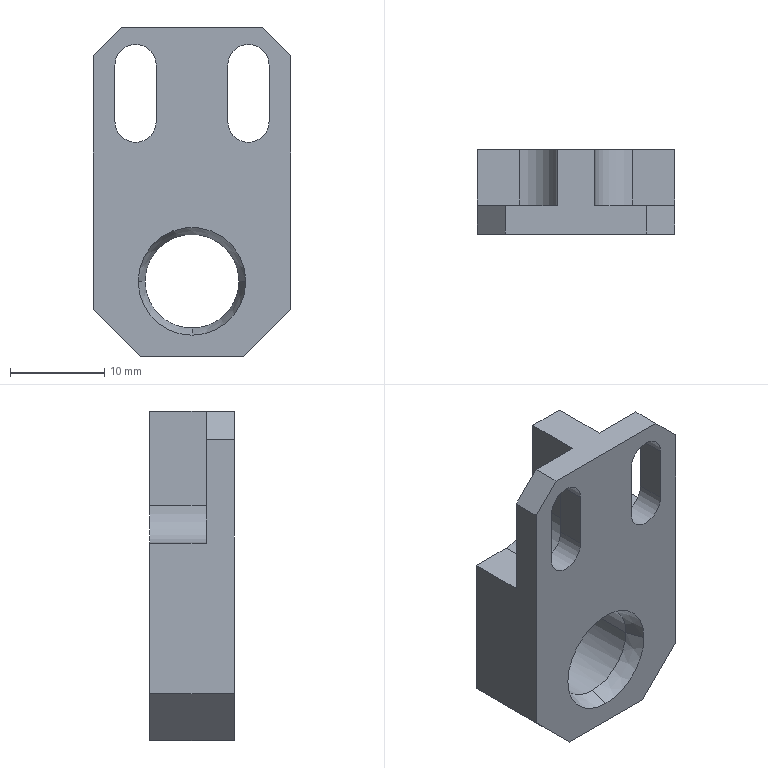Part | STEP file | 1519D1D1-5.stp.STEP | 1 solid | 31 faces | box 21 x 9 x 35 mm | volume 3996 mm3 | plane 20 | cylinder 8 | cone 3 | commonest cylinder face diameters 4.4 x4 8 x2 10 x2
STEP:
#1=CARTESIAN_POINT('',(-8.2,0.,-10.));
#2=VERTEX_POINT('',#1);
#3=CARTESIAN_POINT('',(-8.2,0.,-4.));
#4=VERTEX_POINT('',#3);
#5=CARTESIAN_POINT('',(-8.2,0.,-10.));
#6=DIRECTION('',(0.,0.,1.));
#7=VECTOR('',#6,1000.);
#8=LINE('',#5,#7);
#9=EDGE_CURVE('',#2,#4,#8,.T.);
#10=ORIENTED_EDGE('',*,*,#9,.T.);
#11=CARTESIAN_POINT('',(-3.8,0.,-4.));
#12=VERTEX_POINT('',#11);
#13=CARTESIAN_POINT('',(-6.,0.,-4.));
#14=DIRECTION('',(0.,1.,0.));
#15=DIRECTION('',(-1.,0.,0.));
#16=AXIS2_PLACEMENT_3D('',#13,#14,#15);
#17=CIRCLE('',#16,2.2);
#18=EDGE_CURVE('',#4,#12,#17,.T.);
#19=ORIENTED_EDGE('',*,*,#18,.T.);
#20=CARTESIAN_POINT('',(-3.8,0.,-10.));
#21=VERTEX_POINT('',#20);
#22=CARTESIAN_POINT('',(-3.8,0.,-4.));
#23=DIRECTION('',(0.,0.,-1.));
#24=VECTOR('',#23,1000.);
#25=LINE('',#22,#24);
#26=EDGE_CURVE('',#12,#21,#25,.T.);
#27=ORIENTED_EDGE('',*,*,#26,.T.);
#28=CARTESIAN_POINT('',(-6.,0.,-10.));
#29=DIRECTION('',(0.,1.,0.));
#30=DIRECTION('',(1.,0.,0.));
#31=AXIS2_PLACEMENT_3D('',#28,#29,#30);
#32=CIRCLE('',#31,2.2);
#33=EDGE_CURVE('',#21,#2,#32,.T.);
#34=ORIENTED_EDGE('',*,*,#33,.T.);
#35=EDGE_LOOP('',(#10,#19,#27,#34));
#36=FACE_BOUND('',#35,.T.);
#37=CARTESIAN_POINT('',(5.728,0.,-27.));
#38=VERTEX_POINT('',#37);
#39=CARTESIAN_POINT('',(0.,0.,-32.728));
#40=VERTEX_POINT('',#39);
#41=CARTESIAN_POINT('',(0.,0.,-27.));
#42=DIRECTION('',(0.,1.,0.));
#43=DIRECTION('',(1.,0.,0.));
#44=AXIS2_PLACEMENT_3D('',#41,#42,#43);
#45=CIRCLE('',#44,5.728);
#46=EDGE_CURVE('',#38,#40,#45,.T.);
#47=ORIENTED_EDGE('',*,*,#46,.T.);
#48=CARTESIAN_POINT('',(-5.728,0.,-27.));
#49=VERTEX_POINT('',#48);
#50=CARTESIAN_POINT('',(0.,0.,-27.));
#51=DIRECTION('',(0.,1.,0.));
#52=DIRECTION('',(1.,0.,0.));
#53=AXIS2_PLACEMENT_3D('',#50,#51,#52);
#54=CIRCLE('',#53,5.728);
#55=EDGE_CURVE('',#40,#49,#54,.T.);
#56=ORIENTED_EDGE('',*,*,#55,.T.);
#57=CARTESIAN_POINT('',(0.,0.,-27.));
#58=DIRECTION('',(0.,1.,0.));
#59=DIRECTION('',(-1.,0.,0.));
#60=AXIS2_PLACEMENT_3D('',#57,#58,#59);
#61=CIRCLE('',#60,5.728);
#62=EDGE_CURVE('',#49,#38,#61,.T.);
#63=ORIENTED_EDGE('',*,*,#62,.T.);
#64=EDGE_LOOP('',(#47,#56,#63));
#65=FACE_BOUND('',#64,.T.);
#66=CARTESIAN_POINT('',(3.8,0.,-4.));
#67=VERTEX_POINT('',#66);
#68=CARTESIAN_POINT('',(8.2,0.,-4.));
#69=VERTEX_POINT('',#68);
#70=CARTESIAN_POINT('',(6.,0.,-4.));
#71=DIRECTION('',(0.,1.,0.));
#72=DIRECTION('',(-1.,0.,0.));
#73=AXIS2_PLACEMENT_3D('',#70,#71,#72);
#74=CIRCLE('',#73,2.2);
#75=EDGE_CURVE('',#67,#69,#74,.T.);
#76=ORIENTED_EDGE('',*,*,#75,.T.);
#77=CARTESIAN_POINT('',(8.2,0.,-10.));
#78=VERTEX_POINT('',#77);
#79=CARTESIAN_POINT('',(8.2,0.,-4.));
#80=DIRECTION('',(0.,0.,-1.));
#81=VECTOR('',#80,1000.);
#82=LINE('',#79,#81);
#83=EDGE_CURVE('',#69,#78,#82,.T.);
#84=ORIENTED_EDGE('',*,*,#83,.T.);
#85=CARTESIAN_POINT('',(3.8,0.,-10.));
#86=VERTEX_POINT('',#85);
#87=CARTESIAN_POINT('',(6.,0.,-10.));
#88=DIRECTION('',(0.,1.,0.));
#89=DIRECTION('',(1.,0.,0.));
#90=AXIS2_PLACEMENT_3D('',#87,#88,#89);
#91=CIRCLE('',#90,2.2);
#92=EDGE_CURVE('',#78,#86,#91,.T.);
#93=ORIENTED_EDGE('',*,*,#92,.T.);
#94=CARTESIAN_POINT('',(3.8,0.,-10.));
#95=DIRECTION('',(0.,0.,1.));
#96=VECTOR('',#95,1000.);
#97=LINE('',#94,#96);
#98=EDGE_CURVE('',#86,#67,#97,.T.);
#99=ORIENTED_EDGE('',*,*,#98,.T.);
#100=EDGE_LOOP('',(#76,#84,#93,#99));
#101=FACE_BOUND('',#100,.T.);
#102=CARTESIAN_POINT('',(5.5,0.,-35.));
#103=VERTEX_POINT('',#102);
#104=CARTESIAN_POINT('',(-5.5,0.,-35.));
#105=VERTEX_POINT('',#104);
#106=CARTESIAN_POINT('',(5.5,0.,-35.));
#107=DIRECTION('',(-1.,0.,0.));
#108=VECTOR('',#107,1000.);
#109=LINE('',#106,#108);
#110=EDGE_CURVE('',#103,#105,#109,.T.);
#111=ORIENTED_EDGE('',*,*,#110,.F.);
#112=CARTESIAN_POINT('',(10.5,0.,-30.));
#113=VERTEX_POINT('',#112);
#114=CARTESIAN_POINT('',(5.5,0.,-35.));
#115=DIRECTION('',(0.7071,0.,0.7071));
#116=VECTOR('',#115,1000.);
#117=LINE('',#114,#116);
#118=EDGE_CURVE('',#103,#113,#117,.T.);
#119=ORIENTED_EDGE('',*,*,#118,.T.);
#120=CARTESIAN_POINT('',(10.5,0.,-3.));
#121=VERTEX_POINT('',#120);
#122=CARTESIAN_POINT('',(10.5,0.,-3.));
#123=DIRECTION('',(0.,0.,-1.));
#124=VECTOR('',#123,1000.);
#125=LINE('',#122,#124);
#126=EDGE_CURVE('',#121,#113,#125,.T.);
#127=ORIENTED_EDGE('',*,*,#126,.F.);
#128=CARTESIAN_POINT('',(7.5,0.,0.));
#129=VERTEX_POINT('',#128);
#130=CARTESIAN_POINT('',(10.5,0.,-3.));
#131=DIRECTION('',(-0.7071,0.,0.7071));
#132=VECTOR('',#131,1000.);
#133=LINE('',#130,#132);
#134=EDGE_CURVE('',#121,#129,#133,.T.);
#135=ORIENTED_EDGE('',*,*,#134,.T.);
#136=CARTESIAN_POINT('',(-7.5,0.,0.));
#137=VERTEX_POINT('',#136);
#138=CARTESIAN_POINT('',(-7.5,0.,0.));
#139=DIRECTION('',(1.,0.,0.));
#140=VECTOR('',#139,1000.);
#141=LINE('',#138,#140);
#142=EDGE_CURVE('',#137,#129,#141,.T.);
#143=ORIENTED_EDGE('',*,*,#142,.F.);
#144=CARTESIAN_POINT('',(-10.5,0.,-3.));
#145=VERTEX_POINT('',#144);
#146=CARTESIAN_POINT('',(-7.5,0.,0.));
#147=DIRECTION('',(-0.7071,0.,-0.7071));
#148=VECTOR('',#147,1000.);
#149=LINE('',#146,#148);
#150=EDGE_CURVE('',#137,#145,#149,.T.);
#151=ORIENTED_EDGE('',*,*,#150,.T.);
#152=CARTESIAN_POINT('',(-10.5,0.,-30.));
#153=VERTEX_POINT('',#152);
#154=CARTESIAN_POINT('',(-10.5,0.,-30.));
#155=DIRECTION('',(0.,0.,1.));
#156=VECTOR('',#155,1000.);
#157=LINE('',#154,#156);
#158=EDGE_CURVE('',#153,#145,#157,.T.);
#159=ORIENTED_EDGE('',*,*,#158,.F.);
#160=CARTESIAN_POINT('',(-10.5,0.,-30.));
#161=DIRECTION('',(0.7071,0.,-0.7071));
#162=VECTOR('',#161,1000.);
#163=LINE('',#160,#162);
#164=EDGE_CURVE('',#153,#105,#163,.T.);
#165=ORIENTED_EDGE('',*,*,#164,.T.);
#166=EDGE_LOOP('',(#111,#119,#127,#135,#143,#151,#159,#165));
#167=FACE_OUTER_BOUND('',#166,.T.);
#168=CARTESIAN_POINT('',(0.,0.,0.));
#169=DIRECTION('',(0.,1.,0.));
#170=DIRECTION('',(1.,0.,0.));
#171=AXIS2_PLACEMENT_3D('',#168,#169,#170);
#172=PLANE('',#171);
#173=ADVANCED_FACE('',(#36,#65,#101,#167),#172,.F.);
#174=CARTESIAN_POINT('',(3.8,3.,-4.));
#175=VERTEX_POINT('',#174);
#176=CARTESIAN_POINT('',(3.8,3.,-4.));
#177=DIRECTION('',(0.,-1.,0.));
#178=VECTOR('',#177,1000.);
#179=LINE('',#176,#178);
#180=EDGE_CURVE('',#175,#67,#179,.T.);
#181=ORIENTED_EDGE('',*,*,#180,.T.);
#182=ORIENTED_EDGE('',*,*,#98,.F.);
#183=CARTESIAN_POINT('',(3.8,3.,-10.));
#184=VERTEX_POINT('',#183);
#185=CARTESIAN_POINT('',(3.8,3.,-10.));
#186=DIRECTION('',(0.,-1.,0.));
#187=VECTOR('',#186,1000.);
#188=LINE('',#185,#187);
#189=EDGE_CURVE('',#184,#86,#188,.T.);
#190=ORIENTED_EDGE('',*,*,#189,.F.);
#191=CARTESIAN_POINT('',(3.8,3.,-10.));
#192=DIRECTION('',(0.,0.,1.));
#193=VECTOR('',#192,1000.);
#194=LINE('',#191,#193);
#195=EDGE_CURVE('',#184,#175,#194,.T.);
#196=ORIENTED_EDGE('',*,*,#195,.T.);
#197=EDGE_LOOP('',(#181,#182,#190,#196));
#198=FACE_OUTER_BOUND('',#197,.T.);
#199=CARTESIAN_POINT('',(3.8,9.,-10.));
#200=DIRECTION('',(-1.,0.,0.));
#201=DIRECTION('',(0.,0.,1.));
#202=AXIS2_PLACEMENT_3D('',#199,#200,#201);
#203=PLANE('',#202);
#204=ADVANCED_FACE('',(#198),#203,.F.);
#205=CARTESIAN_POINT('',(-3.8,3.,-4.));
#206=VERTEX_POINT('',#205);
#207=CARTESIAN_POINT('',(-3.8,3.,-10.));
#208=VERTEX_POINT('',#207);
#209=CARTESIAN_POINT('',(-3.8,3.,-4.));
#210=DIRECTION('',(0.,0.,-1.));
#211=VECTOR('',#210,1000.);
#212=LINE('',#209,#211);
#213=EDGE_CURVE('',#206,#208,#212,.T.);
#214=ORIENTED_EDGE('',*,*,#213,.F.);
#215=CARTESIAN_POINT('',(-8.2,3.,-4.));
#216=VERTEX_POINT('',#215);
#217=CARTESIAN_POINT('',(-6.,3.,-4.));
#218=DIRECTION('',(0.,1.,0.));
#219=DIRECTION('',(-1.,0.,0.));
#220=AXIS2_PLACEMENT_3D('',#217,#218,#219);
#221=CIRCLE('',#220,2.2);
#222=EDGE_CURVE('',#216,#206,#221,.T.);
#223=ORIENTED_EDGE('',*,*,#222,.F.);
#224=CARTESIAN_POINT('',(-8.2,3.,-10.));
#225=VERTEX_POINT('',#224);
#226=CARTESIAN_POINT('',(-8.2,3.,-10.));
#227=DIRECTION('',(0.,0.,1.));
#228=VECTOR('',#227,1000.);
#229=LINE('',#226,#228);
#230=EDGE_CURVE('',#225,#216,#229,.T.);
#231=ORIENTED_EDGE('',*,*,#230,.F.);
#232=CARTESIAN_POINT('',(-6.,3.,-10.));
#233=DIRECTION('',(0.,1.,0.));
#234=DIRECTION('',(1.,0.,0.));
#235=AXIS2_PLACEMENT_3D('',#232,#233,#234);
#236=CIRCLE('',#235,2.2);
#237=EDGE_CURVE('',#208,#225,#236,.T.);
#238=ORIENTED_EDGE('',*,*,#237,.F.);
#239=EDGE_LOOP('',(#214,#223,#231,#238));
#240=FACE_BOUND('',#239,.T.);
#241=CARTESIAN_POINT('',(-7.5,3.,0.));
#242=VERTEX_POINT('',#241);
#243=CARTESIAN_POINT('',(-2.,3.,0.));
#244=VERTEX_POINT('',#243);
#245=CARTESIAN_POINT('',(-7.5,3.,0.));
#246=DIRECTION('',(1.,0.,0.));
#247=VECTOR('',#246,1000.);
#248=LINE('',#245,#247);
#249=EDGE_CURVE('',#242,#244,#248,.T.);
#250=ORIENTED_EDGE('',*,*,#249,.T.);
#251=CARTESIAN_POINT('',(-2.,3.,-10.));
#252=VERTEX_POINT('',#251);
#253=CARTESIAN_POINT('',(-2.,3.,0.));
#254=DIRECTION('',(0.,0.,-1.));
#255=VECTOR('',#254,1000.);
#256=LINE('',#253,#255);
#257=EDGE_CURVE('',#244,#252,#256,.T.);
#258=ORIENTED_EDGE('',*,*,#257,.T.);
#259=CARTESIAN_POINT('',(-6.,3.,-14.));
#260=VERTEX_POINT('',#259);
#261=CARTESIAN_POINT('',(-6.,3.,-10.));
#262=DIRECTION('',(0.,1.,0.));
#263=DIRECTION('',(1.,0.,0.));
#264=AXIS2_PLACEMENT_3D('',#261,#262,#263);
#265=CIRCLE('',#264,4.);
#266=EDGE_CURVE('',#252,#260,#265,.T.);
#267=ORIENTED_EDGE('',*,*,#266,.T.);
#268=CARTESIAN_POINT('',(-10.5,3.,-14.));
#269=VERTEX_POINT('',#268);
#270=CARTESIAN_POINT('',(-6.,3.,-14.));
#271=DIRECTION('',(-1.,0.,0.));
#272=VECTOR('',#271,1000.);
#273=LINE('',#270,#272);
#274=EDGE_CURVE('',#260,#269,#273,.T.);
#275=ORIENTED_EDGE('',*,*,#274,.T.);
#276=CARTESIAN_POINT('',(-10.5,3.,-3.));
#277=VERTEX_POINT('',#276);
#278=CARTESIAN_POINT('',(-10.5,3.,-3.));
#279=DIRECTION('',(0.,0.,-1.));
#280=VECTOR('',#279,1000.);
#281=LINE('',#278,#280);
#282=EDGE_CURVE('',#277,#269,#281,.T.);
#283=ORIENTED_EDGE('',*,*,#282,.F.);
#284=CARTESIAN_POINT('',(-10.5,3.,-3.));
#285=DIRECTION('',(0.7071,0.,0.7071));
#286=VECTOR('',#285,1000.);
#287=LINE('',#284,#286);
#288=EDGE_CURVE('',#277,#242,#287,.T.);
#289=ORIENTED_EDGE('',*,*,#288,.T.);
#290=EDGE_LOOP('',(#250,#258,#267,#275,#283,#289));
#291=FACE_OUTER_BOUND('',#290,.T.);
#292=CARTESIAN_POINT('',(0.,3.,0.));
#293=DIRECTION('',(0.,1.,0.));
#294=DIRECTION('',(1.,0.,0.));
#295=AXIS2_PLACEMENT_3D('',#292,#293,#294);
#296=PLANE('',#295);
#297=ADVANCED_FACE('',(#240,#291),#296,.T.);
#298=CARTESIAN_POINT('',(8.2,3.,-10.));
#299=VERTEX_POINT('',#298);
#300=CARTESIAN_POINT('',(6.,3.,-10.));
#301=DIRECTION('',(0.,1.,0.));
#302=DIRECTION('',(1.,0.,0.));
#303=AXIS2_PLACEMENT_3D('',#300,#301,#302);
#304=CIRCLE('',#303,2.2);
#305=EDGE_CURVE('',#299,#184,#304,.T.);
#306=ORIENTED_EDGE('',*,*,#305,.F.);
#307=CARTESIAN_POINT('',(8.2,3.,-4.));
#308=VERTEX_POINT('',#307);
#309=CARTESIAN_POINT('',(8.2,3.,-4.));
#310=DIRECTION('',(0.,0.,-1.));
#311=VECTOR('',#310,1000.);
#312=LINE('',#309,#311);
#313=EDGE_CURVE('',#308,#299,#312,.T.);
#314=ORIENTED_EDGE('',*,*,#313,.F.);
#315=CARTESIAN_POINT('',(6.,3.,-4.));
#316=DIRECTION('',(0.,1.,0.));
#317=DIRECTION('',(-1.,0.,0.));
#318=AXIS2_PLACEMENT_3D('',#315,#316,#317);
#319=CIRCLE('',#318,2.2);
#320=EDGE_CURVE('',#175,#308,#319,.T.);
#321=ORIENTED_EDGE('',*,*,#320,.F.);
#322=ORIENTED_EDGE('',*,*,#195,.F.);
#323=EDGE_LOOP('',(#306,#314,#321,#322));
#324=FACE_BOUND('',#323,.T.);
#325=CARTESIAN_POINT('',(10.5,3.,-3.));
#326=VERTEX_POINT('',#325);
#327=CARTESIAN_POINT('',(10.5,3.,-14.));
#328=VERTEX_POINT('',#327);
#329=CARTESIAN_POINT('',(10.5,3.,-3.));
#330=DIRECTION('',(0.,0.,-1.));
#331=VECTOR('',#330,1000.);
#332=LINE('',#329,#331);
#333=EDGE_CURVE('',#326,#328,#332,.T.);
#334=ORIENTED_EDGE('',*,*,#333,.T.);
#335=CARTESIAN_POINT('',(6.,3.,-14.));
#336=VERTEX_POINT('',#335);
#337=CARTESIAN_POINT('',(10.5,3.,-14.));
#338=DIRECTION('',(-1.,0.,0.));
#339=VECTOR('',#338,1000.);
#340=LINE('',#337,#339);
#341=EDGE_CURVE('',#328,#336,#340,.T.);
#342=ORIENTED_EDGE('',*,*,#341,.T.);
#343=CARTESIAN_POINT('',(2.,3.,-10.));
#344=VERTEX_POINT('',#343);
#345=CARTESIAN_POINT('',(6.,3.,-10.));
#346=DIRECTION('',(0.,1.,0.));
#347=DIRECTION('',(0.,0.,-1.));
#348=AXIS2_PLACEMENT_3D('',#345,#346,#347);
#349=CIRCLE('',#348,4.);
#350=EDGE_CURVE('',#336,#344,#349,.T.);
#351=ORIENTED_EDGE('',*,*,#350,.T.);
#352=CARTESIAN_POINT('',(2.,3.,0.));
#353=VERTEX_POINT('',#352);
#354=CARTESIAN_POINT('',(2.,3.,-10.));
#355=DIRECTION('',(0.,0.,1.));
#356=VECTOR('',#355,1000.);
#357=LINE('',#354,#356);
#358=EDGE_CURVE('',#344,#353,#357,.T.);
#359=ORIENTED_EDGE('',*,*,#358,.T.);
#360=CARTESIAN_POINT('',(7.5,3.,0.));
#361=VERTEX_POINT('',#360);
#362=CARTESIAN_POINT('',(2.,3.,0.));
#363=DIRECTION('',(1.,0.,0.));
#364=VECTOR('',#363,1000.);
#365=LINE('',#362,#364);
#366=EDGE_CURVE('',#353,#361,#365,.T.);
#367=ORIENTED_EDGE('',*,*,#366,.T.);
#368=CARTESIAN_POINT('',(7.5,3.,0.));
#369=DIRECTION('',(0.7071,0.,-0.7071));
#370=VECTOR('',#369,1000.);
#371=LINE('',#368,#370);
#372=EDGE_CURVE('',#361,#326,#371,.T.);
#373=ORIENTED_EDGE('',*,*,#372,.T.);
#374=EDGE_LOOP('',(#334,#342,#351,#359,#367,#373));
#375=FACE_OUTER_BOUND('',#374,.T.);
#376=CARTESIAN_POINT('',(0.,3.,0.));
#377=DIRECTION('',(0.,1.,0.));
#378=DIRECTION('',(1.,0.,0.));
#379=AXIS2_PLACEMENT_3D('',#376,#377,#378);
#380=PLANE('',#379);
#381=ADVANCED_FACE('',(#324,#375),#380,.T.);
#382=CARTESIAN_POINT('',(-8.2,3.,-10.));
#383=DIRECTION('',(0.,-1.,0.));
#384=VECTOR('',#383,1000.);
#385=LINE('',#382,#384);
#386=EDGE_CURVE('',#225,#2,#385,.T.);
#387=ORIENTED_EDGE('',*,*,#386,.T.);
#388=ORIENTED_EDGE('',*,*,#33,.F.);
#389=CARTESIAN_POINT('',(-3.8,3.,-10.));
#390=DIRECTION('',(0.,-1.,0.));
#391=VECTOR('',#390,1000.);
#392=LINE('',#389,#391);
#393=EDGE_CURVE('',#208,#21,#392,.T.);
#394=ORIENTED_EDGE('',*,*,#393,.F.);
#395=ORIENTED_EDGE('',*,*,#237,.T.);
#396=EDGE_LOOP('',(#387,#388,#394,#395));
#397=FACE_OUTER_BOUND('',#396,.T.);
#398=CARTESIAN_POINT('',(-6.,9.,-10.));
#399=DIRECTION('',(0.,1.,0.));
#400=DIRECTION('',(1.,0.,0.));
#401=AXIS2_PLACEMENT_3D('',#398,#399,#400);
#402=CYLINDRICAL_SURFACE('',#401,2.2);
#403=ADVANCED_FACE('',(#397),#402,.F.);
#404=ORIENTED_EDGE('',*,*,#393,.T.);
#405=ORIENTED_EDGE('',*,*,#26,.F.);
#406=CARTESIAN_POINT('',(-3.8,3.,-4.));
#407=DIRECTION('',(0.,-1.,0.));
#408=VECTOR('',#407,1000.);
#409=LINE('',#406,#408);
#410=EDGE_CURVE('',#206,#12,#409,.T.);
#411=ORIENTED_EDGE('',*,*,#410,.F.);
#412=ORIENTED_EDGE('',*,*,#213,.T.);
#413=EDGE_LOOP('',(#404,#405,#411,#412));
#414=FACE_OUTER_BOUND('',#413,.T.);
#415=CARTESIAN_POINT('',(-3.8,9.,-4.));
#416=DIRECTION('',(1.,0.,0.));
#417=DIRECTION('',(0.,1.,0.));
#418=AXIS2_PLACEMENT_3D('',#415,#416,#417);
#419=PLANE('',#418);
#420=ADVANCED_FACE('',(#414),#419,.F.);
#421=ORIENTED_EDGE('',*,*,#410,.T.);
#422=ORIENTED_EDGE('',*,*,#18,.F.);
#423=CARTESIAN_POINT('',(-8.2,3.,-4.));
#424=DIRECTION('',(0.,-1.,0.));
#425=VECTOR('',#424,1000.);
#426=LINE('',#423,#425);
#427=EDGE_CURVE('',#216,#4,#426,.T.);
#428=ORIENTED_EDGE('',*,*,#427,.F.);
#429=ORIENTED_EDGE('',*,*,#222,.T.);
#430=EDGE_LOOP('',(#421,#422,#428,#429));
#431=FACE_OUTER_BOUND('',#430,.T.);
#432=CARTESIAN_POINT('',(-6.,9.,-4.));
#433=DIRECTION('',(0.,1.,0.));
#434=DIRECTION('',(1.,0.,0.));
#435=AXIS2_PLACEMENT_3D('',#432,#433,#434);
#436=CYLINDRICAL_SURFACE('',#435,2.2);
#437=ADVANCED_FACE('',(#431),#436,.F.);
#438=ORIENTED_EDGE('',*,*,#427,.T.);
#439=ORIENTED_EDGE('',*,*,#9,.F.);
#440=ORIENTED_EDGE('',*,*,#386,.F.);
#441=ORIENTED_EDGE('',*,*,#230,.T.);
#442=EDGE_LOOP('',(#438,#439,#440,#441));
#443=FACE_OUTER_BOUND('',#442,.T.);
#444=CARTESIAN_POINT('',(-8.2,9.,-10.));
#445=DIRECTION('',(-1.,0.,0.));
#446=DIRECTION('',(0.,0.,1.));
#447=AXIS2_PLACEMENT_3D('',#444,#445,#446);
#448=PLANE('',#447);
#449=ADVANCED_FACE('',(#443),#448,.F.);
#450=CARTESIAN_POINT('',(8.2,3.,-4.));
#451=DIRECTION('',(0.,-1.,0.));
#452=VECTOR('',#451,1000.);
#453=LINE('',#450,#452);
#454=EDGE_CURVE('',#308,#69,#453,.T.);
#455=ORIENTED_EDGE('',*,*,#454,.T.);
#456=ORIENTED_EDGE('',*,*,#75,.F.);
#457=ORIENTED_EDGE('',*,*,#180,.F.);
#458=ORIENTED_EDGE('',*,*,#320,.T.);
#459=EDGE_LOOP('',(#455,#456,#457,#458));
#460=FACE_OUTER_BOUND('',#459,.T.);
#461=CARTESIAN_POINT('',(6.,9.,-4.));
#462=DIRECTION('',(0.,1.,0.));
#463=DIRECTION('',(1.,0.,0.));
#464=AXIS2_PLACEMENT_3D('',#461,#462,#463);
#465=CYLINDRICAL_SURFACE('',#464,2.2);
#466=ADVANCED_FACE('',(#460),#465,.F.);
#467=CARTESIAN_POINT('',(8.2,3.,-10.));
#468=DIRECTION('',(0.,-1.,0.));
#469=VECTOR('',#468,1000.);
#470=LINE('',#467,#469);
#471=EDGE_CURVE('',#299,#78,#470,.T.);
#472=ORIENTED_EDGE('',*,*,#471,.T.);
#473=ORIENTED_EDGE('',*,*,#83,.F.);
#474=ORIENTED_EDGE('',*,*,#454,.F.);
#475=ORIENTED_EDGE('',*,*,#313,.T.);
#476=EDGE_LOOP('',(#472,#473,#474,#475));
#477=FACE_OUTER_BOUND('',#476,.T.);
#478=CARTESIAN_POINT('',(8.2,9.,-4.));
#479=DIRECTION('',(1.,0.,0.));
#480=DIRECTION('',(0.,1.,0.));
#481=AXIS2_PLACEMENT_3D('',#478,#479,#480);
#482=PLANE('',#481);
#483=ADVANCED_FACE('',(#477),#482,.F.);
#484=ORIENTED_EDGE('',*,*,#189,.T.);
#485=ORIENTED_EDGE('',*,*,#92,.F.);
#486=ORIENTED_EDGE('',*,*,#471,.F.);
#487=ORIENTED_EDGE('',*,*,#305,.T.);
#488=EDGE_LOOP('',(#484,#485,#486,#487));
#489=FACE_OUTER_BOUND('',#488,.T.);
#490=CARTESIAN_POINT('',(6.,9.,-10.));
#491=DIRECTION('',(0.,1.,0.));
#492=DIRECTION('',(1.,0.,0.));
#493=AXIS2_PLACEMENT_3D('',#490,#491,#492);
#494=CYLINDRICAL_SURFACE('',#493,2.2);
#495=ADVANCED_FACE('',(#489),#494,.F.);
#496=CARTESIAN_POINT('',(-7.5,3.,0.));
#497=DIRECTION('',(0.,-1.,0.));
#498=VECTOR('',#497,1000.);
#499=LINE('',#496,#498);
#500=EDGE_CURVE('',#242,#137,#499,.T.);
#501=ORIENTED_EDGE('',*,*,#500,.F.);
#502=ORIENTED_EDGE('',*,*,#288,.F.);
#503=CARTESIAN_POINT('',(-10.5,3.,-3.));
#504=DIRECTION('',(0.,-1.,0.));
#505=VECTOR('',#504,1000.);
#506=LINE('',#503,#505);
#507=EDGE_CURVE('',#277,#145,#506,.T.);
#508=ORIENTED_EDGE('',*,*,#507,.T.);
#509=ORIENTED_EDGE('',*,*,#150,.F.);
#510=EDGE_LOOP('',(#501,#502,#508,#509));
#511=FACE_OUTER_BOUND('',#510,.T.);
#512=CARTESIAN_POINT('',(-9.,1.5,-1.5));
#513=DIRECTION('',(-0.7071,0.,0.7071));
#514=DIRECTION('',(0.,1.,0.));
#515=AXIS2_PLACEMENT_3D('',#512,#513,#514);
#516=PLANE('',#515);
#517=ADVANCED_FACE('',(#511),#516,.T.);
#518=ORIENTED_EDGE('',*,*,#158,.T.);
#519=ORIENTED_EDGE('',*,*,#507,.F.);
#520=ORIENTED_EDGE('',*,*,#282,.T.);
#521=CARTESIAN_POINT('',(-10.5,9.,-14.));
#522=VERTEX_POINT('',#521);
#523=CARTESIAN_POINT('',(-10.5,9.,-14.));
#524=DIRECTION('',(0.,-1.,0.));
#525=VECTOR('',#524,1000.);
#526=LINE('',#523,#525);
#527=EDGE_CURVE('',#522,#269,#526,.T.);
#528=ORIENTED_EDGE('',*,*,#527,.F.);
#529=CARTESIAN_POINT('',(-10.5,9.,-30.));
#530=VERTEX_POINT('',#529);
#531=CARTESIAN_POINT('',(-10.5,9.,-30.));
#532=DIRECTION('',(0.,0.,1.));
#533=VECTOR('',#532,1000.);
#534=LINE('',#531,#533);
#535=EDGE_CURVE('',#530,#522,#534,.T.);
#536=ORIENTED_EDGE('',*,*,#535,.F.);
#537=CARTESIAN_POINT('',(-10.5,9.,-30.));
#538=DIRECTION('',(0.,-1.,0.));
#539=VECTOR('',#538,1000.);
#540=LINE('',#537,#539);
#541=EDGE_CURVE('',#530,#153,#540,.T.);
#542=ORIENTED_EDGE('',*,*,#541,.T.);
#543=EDGE_LOOP('',(#518,#519,#520,#528,#536,#542));
#544=FACE_OUTER_BOUND('',#543,.T.);
#545=CARTESIAN_POINT('',(-10.5,0.,-35.));
#546=DIRECTION('',(-1.,0.,0.));
#547=DIRECTION('',(0.,0.,1.));
#548=AXIS2_PLACEMENT_3D('',#545,#546,#547);
#549=PLANE('',#548);
#550=ADVANCED_FACE('',(#544),#549,.T.);
#551=ORIENTED_EDGE('',*,*,#541,.F.);
#552=CARTESIAN_POINT('',(-5.5,9.,-35.));
#553=VERTEX_POINT('',#552);
#554=CARTESIAN_POINT('',(-5.5,9.,-35.));
#555=DIRECTION('',(-0.7071,0.,0.7071));
#556=VECTOR('',#555,1000.);
#557=LINE('',#554,#556);
#558=EDGE_CURVE('',#553,#530,#557,.T.);
#559=ORIENTED_EDGE('',*,*,#558,.F.);
#560=CARTESIAN_POINT('',(-5.5,9.,-35.));
#561=DIRECTION('',(0.,-1.,0.));
#562=VECTOR('',#561,1000.);
#563=LINE('',#560,#562);
#564=EDGE_CURVE('',#553,#105,#563,.T.);
#565=ORIENTED_EDGE('',*,*,#564,.T.);
#566=ORIENTED_EDGE('',*,*,#164,.F.);
#567=EDGE_LOOP('',(#551,#559,#565,#566));
#568=FACE_OUTER_BOUND('',#567,.T.);
#569=CARTESIAN_POINT('',(-8.,4.5,-32.5));
#570=DIRECTION('',(-0.7071,0.,-0.7071));
#571=DIRECTION('',(-0.7071,0.,0.7071));
#572=AXIS2_PLACEMENT_3D('',#569,#570,#571);
#573=PLANE('',#572);
#574=ADVANCED_FACE('',(#568),#573,.T.);
#575=CARTESIAN_POINT('',(5.5,9.,-35.));
#576=VERTEX_POINT('',#575);
#577=CARTESIAN_POINT('',(5.5,9.,-35.));
#578=DIRECTION('',(-1.,0.,0.));
#579=VECTOR('',#578,1000.);
#580=LINE('',#577,#579);
#581=EDGE_CURVE('',#576,#553,#580,.T.);
#582=ORIENTED_EDGE('',*,*,#581,.F.);
#583=CARTESIAN_POINT('',(5.5,9.,-35.));
#584=DIRECTION('',(0.,-1.,0.));
#585=VECTOR('',#584,1000.);
#586=LINE('',#583,#585);
#587=EDGE_CURVE('',#576,#103,#586,.T.);
#588=ORIENTED_EDGE('',*,*,#587,.T.);
#589=ORIENTED_EDGE('',*,*,#110,.T.);
#590=ORIENTED_EDGE('',*,*,#564,.F.);
#591=EDGE_LOOP('',(#582,#588,#589,#590));
#592=FACE_OUTER_BOUND('',#591,.T.);
#593=CARTESIAN_POINT('',(10.5,0.,-35.));
#594=DIRECTION('',(0.,0.,-1.));
#595=DIRECTION('',(0.,-1.,0.));
#596=AXIS2_PLACEMENT_3D('',#593,#594,#595);
#597=PLANE('',#596);
#598=ADVANCED_FACE('',(#592),#597,.T.);
#599=ORIENTED_EDGE('',*,*,#587,.F.);
#600=CARTESIAN_POINT('',(10.5,9.,-30.));
#601=VERTEX_POINT('',#600);
#602=CARTESIAN_POINT('',(10.5,9.,-30.));
#603=DIRECTION('',(-0.7071,0.,-0.7071));
#604=VECTOR('',#603,1000.);
#605=LINE('',#602,#604);
#606=EDGE_CURVE('',#601,#576,#605,.T.);
#607=ORIENTED_EDGE('',*,*,#606,.F.);
#608=CARTESIAN_POINT('',(10.5,9.,-30.));
#609=DIRECTION('',(0.,-1.,0.));
#610=VECTOR('',#609,1000.);
#611=LINE('',#608,#610);
#612=EDGE_CURVE('',#601,#113,#611,.T.);
#613=ORIENTED_EDGE('',*,*,#612,.T.);
#614=ORIENTED_EDGE('',*,*,#118,.F.);
#615=EDGE_LOOP('',(#599,#607,#613,#614));
#616=FACE_OUTER_BOUND('',#615,.T.);
#617=CARTESIAN_POINT('',(8.,4.5,-32.5));
#618=DIRECTION('',(0.7071,0.,-0.7071));
#619=DIRECTION('',(0.,-1.,0.));
#620=AXIS2_PLACEMENT_3D('',#617,#618,#619);
#621=PLANE('',#620);
#622=ADVANCED_FACE('',(#616),#621,.T.);
#623=CARTESIAN_POINT('',(10.5,9.,-14.));
#624=VERTEX_POINT('',#623);
#625=CARTESIAN_POINT('',(10.5,9.,-14.));
#626=DIRECTION('',(0.,0.,-1.));
#627=VECTOR('',#626,1000.);
#628=LINE('',#625,#627);
#629=EDGE_CURVE('',#624,#601,#628,.T.);
#630=ORIENTED_EDGE('',*,*,#629,.F.);
#631=CARTESIAN_POINT('',(10.5,9.,-14.));
#632=DIRECTION('',(0.,-1.,0.));
#633=VECTOR('',#632,1000.);
#634=LINE('',#631,#633);
#635=EDGE_CURVE('',#624,#328,#634,.T.);
#636=ORIENTED_EDGE('',*,*,#635,.T.);
#637=ORIENTED_EDGE('',*,*,#333,.F.);
#638=CARTESIAN_POINT('',(10.5,3.,-3.));
#639=DIRECTION('',(0.,-1.,0.));
#640=VECTOR('',#639,1000.);
#641=LINE('',#638,#640);
#642=EDGE_CURVE('',#326,#121,#641,.T.);
#643=ORIENTED_EDGE('',*,*,#642,.T.);
#644=ORIENTED_EDGE('',*,*,#126,.T.);
#645=ORIENTED_EDGE('',*,*,#612,.F.);
#646=EDGE_LOOP('',(#630,#636,#637,#643,#644,#645));
#647=FACE_OUTER_BOUND('',#646,.T.);
#648=CARTESIAN_POINT('',(10.5,0.,0.));
#649=DIRECTION('',(1.,0.,0.));
#650=DIRECTION('',(0.,1.,0.));
#651=AXIS2_PLACEMENT_3D('',#648,#649,#650);
#652=PLANE('',#651);
#653=ADVANCED_FACE('',(#647),#652,.T.);
#654=ORIENTED_EDGE('',*,*,#642,.F.);
#655=ORIENTED_EDGE('',*,*,#372,.F.);
#656=CARTESIAN_POINT('',(7.5,3.,0.));
#657=DIRECTION('',(0.,-1.,0.));
#658=VECTOR('',#657,1000.);
#659=LINE('',#656,#658);
#660=EDGE_CURVE('',#361,#129,#659,.T.);
#661=ORIENTED_EDGE('',*,*,#660,.T.);
#662=ORIENTED_EDGE('',*,*,#134,.F.);
#663=EDGE_LOOP('',(#654,#655,#661,#662));
#664=FACE_OUTER_BOUND('',#663,.T.);
#665=CARTESIAN_POINT('',(9.,1.5,-1.5));
#666=DIRECTION('',(0.7071,0.,0.7071));
#667=DIRECTION('',(0.,-1.,0.));
#668=AXIS2_PLACEMENT_3D('',#665,#666,#667);
#669=PLANE('',#668);
#670=ADVANCED_FACE('',(#664),#669,.T.);
#671=ORIENTED_EDGE('',*,*,#142,.T.);
#672=ORIENTED_EDGE('',*,*,#660,.F.);
#673=ORIENTED_EDGE('',*,*,#366,.F.);
#674=CARTESIAN_POINT('',(2.,9.,0.));
#675=VERTEX_POINT('',#674);
#676=CARTESIAN_POINT('',(2.,9.,0.));
#677=DIRECTION('',(0.,-1.,0.));
#678=VECTOR('',#677,1000.);
#679=LINE('',#676,#678);
#680=EDGE_CURVE('',#675,#353,#679,.T.);
#681=ORIENTED_EDGE('',*,*,#680,.F.);
#682=CARTESIAN_POINT('',(-2.,9.,0.));
#683=VERTEX_POINT('',#682);
#684=CARTESIAN_POINT('',(-2.,9.,0.));
#685=DIRECTION('',(1.,0.,0.));
#686=VECTOR('',#685,1000.);
#687=LINE('',#684,#686);
#688=EDGE_CURVE('',#683,#675,#687,.T.);
#689=ORIENTED_EDGE('',*,*,#688,.F.);
#690=CARTESIAN_POINT('',(-2.,9.,0.));
#691=DIRECTION('',(0.,-1.,0.));
#692=VECTOR('',#691,1000.);
#693=LINE('',#690,#692);
#694=EDGE_CURVE('',#683,#244,#693,.T.);
#695=ORIENTED_EDGE('',*,*,#694,.T.);
#696=ORIENTED_EDGE('',*,*,#249,.F.);
#697=ORIENTED_EDGE('',*,*,#500,.T.);
#698=EDGE_LOOP('',(#671,#672,#673,#681,#689,#695,#696,#697));
#699=FACE_OUTER_BOUND('',#698,.T.);
#700=CARTESIAN_POINT('',(-10.5,0.,0.));
#701=DIRECTION('',(0.,0.,1.));
#702=DIRECTION('',(1.,0.,0.));
#703=AXIS2_PLACEMENT_3D('',#700,#701,#702);
#704=PLANE('',#703);
#705=ADVANCED_FACE('',(#699),#704,.T.);
#706=CARTESIAN_POINT('',(-2.,9.,-10.));
#707=VERTEX_POINT('',#706);
#708=CARTESIAN_POINT('',(-2.,9.,-10.));
#709=DIRECTION('',(0.,-1.,0.));
#710=VECTOR('',#709,1000.);
#711=LINE('',#708,#710);
#712=EDGE_CURVE('',#707,#252,#711,.T.);
#713=ORIENTED_EDGE('',*,*,#712,.T.);
#714=ORIENTED_EDGE('',*,*,#257,.F.);
#715=ORIENTED_EDGE('',*,*,#694,.F.);
#716=CARTESIAN_POINT('',(-2.,9.,0.));
#717=DIRECTION('',(0.,0.,-1.));
#718=VECTOR('',#717,1000.);
#719=LINE('',#716,#718);
#720=EDGE_CURVE('',#683,#707,#719,.T.);
#721=ORIENTED_EDGE('',*,*,#720,.T.);
#722=EDGE_LOOP('',(#713,#714,#715,#721));
#723=FACE_OUTER_BOUND('',#722,.T.);
#724=CARTESIAN_POINT('',(-2.,9.,0.));
#725=DIRECTION('',(1.,0.,0.));
#726=DIRECTION('',(0.,1.,0.));
#727=AXIS2_PLACEMENT_3D('',#724,#725,#726);
#728=PLANE('',#727);
#729=ADVANCED_FACE('',(#723),#728,.F.);
#730=CARTESIAN_POINT('',(-5.,9.,-27.));
#731=VERTEX_POINT('',#730);
#732=CARTESIAN_POINT('',(5.,9.,-27.));
#733=VERTEX_POINT('',#732);
#734=CARTESIAN_POINT('',(0.,9.,-27.));
#735=DIRECTION('',(0.,1.,0.));
#736=DIRECTION('',(-1.,0.,0.));
#737=AXIS2_PLACEMENT_3D('',#734,#735,#736);
#738=CIRCLE('',#737,5.);
#739=EDGE_CURVE('',#731,#733,#738,.T.);
#740=ORIENTED_EDGE('',*,*,#739,.F.);
#741=CARTESIAN_POINT('',(0.,9.,-27.));
#742=DIRECTION('',(0.,1.,0.));
#743=DIRECTION('',(1.,0.,0.));
#744=AXIS2_PLACEMENT_3D('',#741,#742,#743);
#745=CIRCLE('',#744,5.);
#746=EDGE_CURVE('',#733,#731,#745,.T.);
#747=ORIENTED_EDGE('',*,*,#746,.F.);
#748=EDGE_LOOP('',(#740,#747));
#749=FACE_BOUND('',#748,.T.);
#750=ORIENTED_EDGE('',*,*,#535,.T.);
#751=CARTESIAN_POINT('',(-6.,9.,-14.));
#752=VERTEX_POINT('',#751);
#753=CARTESIAN_POINT('',(-10.5,9.,-14.));
#754=DIRECTION('',(1.,0.,0.));
#755=VECTOR('',#754,1000.);
#756=LINE('',#753,#755);
#757=EDGE_CURVE('',#522,#752,#756,.T.);
#758=ORIENTED_EDGE('',*,*,#757,.T.);
#759=CARTESIAN_POINT('',(-6.,9.,-10.));
#760=DIRECTION('',(0.,1.,0.));
#761=DIRECTION('',(1.,0.,0.));
#762=AXIS2_PLACEMENT_3D('',#759,#760,#761);
#763=CIRCLE('',#762,4.);
#764=EDGE_CURVE('',#707,#752,#763,.T.);
#765=ORIENTED_EDGE('',*,*,#764,.F.);
#766=ORIENTED_EDGE('',*,*,#720,.F.);
#767=ORIENTED_EDGE('',*,*,#688,.T.);
#768=CARTESIAN_POINT('',(2.,9.,-10.));
#769=VERTEX_POINT('',#768);
#770=CARTESIAN_POINT('',(2.,9.,0.));
#771=DIRECTION('',(0.,0.,-1.));
#772=VECTOR('',#771,1000.);
#773=LINE('',#770,#772);
#774=EDGE_CURVE('',#675,#769,#773,.T.);
#775=ORIENTED_EDGE('',*,*,#774,.T.);
#776=CARTESIAN_POINT('',(6.,9.,-14.));
#777=VERTEX_POINT('',#776);
#778=CARTESIAN_POINT('',(6.,9.,-10.));
#779=DIRECTION('',(0.,1.,0.));
#780=DIRECTION('',(0.,0.,-1.));
#781=AXIS2_PLACEMENT_3D('',#778,#779,#780);
#782=CIRCLE('',#781,4.);
#783=EDGE_CURVE('',#777,#769,#782,.T.);
#784=ORIENTED_EDGE('',*,*,#783,.F.);
#785=CARTESIAN_POINT('',(10.5,9.,-14.));
#786=DIRECTION('',(-1.,0.,0.));
#787=VECTOR('',#786,1000.);
#788=LINE('',#785,#787);
#789=EDGE_CURVE('',#624,#777,#788,.T.);
#790=ORIENTED_EDGE('',*,*,#789,.F.);
#791=ORIENTED_EDGE('',*,*,#629,.T.);
#792=ORIENTED_EDGE('',*,*,#606,.T.);
#793=ORIENTED_EDGE('',*,*,#581,.T.);
#794=ORIENTED_EDGE('',*,*,#558,.T.);
#795=EDGE_LOOP('',(#750,#758,#765,#766,#767,#775,#784,#790,#791,#792,#793,#794));
#796=FACE_OUTER_BOUND('',#795,.T.);
#797=CARTESIAN_POINT('',(0.,9.,0.));
#798=DIRECTION('',(0.,1.,0.));
#799=DIRECTION('',(1.,0.,0.));
#800=AXIS2_PLACEMENT_3D('',#797,#798,#799);
#801=PLANE('',#800);
#802=ADVANCED_FACE('',(#749,#796),#801,.T.);
#803=CARTESIAN_POINT('',(5.,2.,-27.));
#804=VERTEX_POINT('',#803);
#805=CARTESIAN_POINT('',(5.,9.,-27.));
#806=DIRECTION('',(0.,-1.,0.));
#807=VECTOR('',#806,1000.);
#808=LINE('',#805,#807);
#809=EDGE_CURVE('',#733,#804,#808,.T.);
#810=ORIENTED_EDGE('',*,*,#809,.F.);
#811=ORIENTED_EDGE('',*,*,#746,.T.);
#812=CARTESIAN_POINT('',(-5.,2.,-27.));
#813=VERTEX_POINT('',#812);
#814=CARTESIAN_POINT('',(-5.,9.,-27.));
#815=DIRECTION('',(0.,-1.,0.));
#816=VECTOR('',#815,1000.);
#817=LINE('',#814,#816);
#818=EDGE_CURVE('',#731,#813,#817,.T.);
#819=ORIENTED_EDGE('',*,*,#818,.T.);
#820=CARTESIAN_POINT('',(0.,2.,-32.));
#821=VERTEX_POINT('',#820);
#822=CARTESIAN_POINT('',(0.,2.,-27.));
#823=DIRECTION('',(0.,1.,0.));
#824=DIRECTION('',(1.,0.,0.));
#825=AXIS2_PLACEMENT_3D('',#822,#823,#824);
#826=CIRCLE('',#825,5.);
#827=EDGE_CURVE('',#821,#813,#826,.T.);
#828=ORIENTED_EDGE('',*,*,#827,.F.);
#829=CARTESIAN_POINT('',(0.,2.,-27.));
#830=DIRECTION('',(0.,1.,0.));
#831=DIRECTION('',(1.,0.,0.));
#832=AXIS2_PLACEMENT_3D('',#829,#830,#831);
#833=CIRCLE('',#832,5.);
#834=EDGE_CURVE('',#804,#821,#833,.T.);
#835=ORIENTED_EDGE('',*,*,#834,.F.);
#836=EDGE_LOOP('',(#810,#811,#819,#828,#835));
#837=FACE_OUTER_BOUND('',#836,.T.);
#838=CARTESIAN_POINT('',(0.,9.,-27.));
#839=DIRECTION('',(0.,1.,0.));
#840=DIRECTION('',(1.,0.,0.));
#841=AXIS2_PLACEMENT_3D('',#838,#839,#840);
#842=CYLINDRICAL_SURFACE('',#841,5.);
#843=ADVANCED_FACE('',(#837),#842,.F.);
#844=CARTESIAN_POINT('',(0.,1.,-32.364));
#845=DIRECTION('',(0.,-0.9397,-0.342));
#846=VECTOR('',#845,1000.);
#847=LINE('',#844,#846);
#848=EDGE_CURVE('',#821,#40,#847,.T.);
#849=ORIENTED_EDGE('',*,*,#848,.F.);
#850=ORIENTED_EDGE('',*,*,#827,.T.);
#851=CARTESIAN_POINT('',(-5.728,0.000000001,-27.));
#852=DIRECTION('',(0.342,0.9397,-0.000000001));
#853=VECTOR('',#852,1000.);
#854=LINE('',#851,#853);
#855=EDGE_CURVE('',#49,#813,#854,.T.);
#856=ORIENTED_EDGE('',*,*,#855,.F.);
#857=ORIENTED_EDGE('',*,*,#55,.F.);
#858=EDGE_LOOP('',(#849,#850,#856,#857));
#859=FACE_OUTER_BOUND('',#858,.T.);
#860=CARTESIAN_POINT('',(0.,1.,-27.));
#861=DIRECTION('',(0.,-1.,0.));
#862=DIRECTION('',(0.,0.,-1.));
#863=AXIS2_PLACEMENT_3D('',#860,#861,#862);
#864=CONICAL_SURFACE('',#863,5.364,0.3491);
#865=ADVANCED_FACE('',(#859),#864,.F.);
#866=ORIENTED_EDGE('',*,*,#855,.T.);
#867=CARTESIAN_POINT('',(0.,2.,-27.));
#868=DIRECTION('',(0.,1.,0.));
#869=DIRECTION('',(-1.,0.,0.));
#870=AXIS2_PLACEMENT_3D('',#867,#868,#869);
#871=CIRCLE('',#870,5.);
#872=EDGE_CURVE('',#813,#804,#871,.T.);
#873=ORIENTED_EDGE('',*,*,#872,.T.);
#874=CARTESIAN_POINT('',(5.728,0.000000001,-27.));
#875=DIRECTION('',(-0.342,0.9397,0.000000001));
#876=VECTOR('',#875,1000.);
#877=LINE('',#874,#876);
#878=EDGE_CURVE('',#38,#804,#877,.T.);
#879=ORIENTED_EDGE('',*,*,#878,.F.);
#880=ORIENTED_EDGE('',*,*,#62,.F.);
#881=EDGE_LOOP('',(#866,#873,#879,#880));
#882=FACE_OUTER_BOUND('',#881,.T.);
#883=CARTESIAN_POINT('',(0.,1.,-27.));
#884=DIRECTION('',(0.,-1.,0.));
#885=DIRECTION('',(0.,0.,-1.));
#886=AXIS2_PLACEMENT_3D('',#883,#884,#885);
#887=CONICAL_SURFACE('',#886,5.364,0.3491);
#888=ADVANCED_FACE('',(#882),#887,.F.);
#889=ORIENTED_EDGE('',*,*,#818,.F.);
#890=ORIENTED_EDGE('',*,*,#739,.T.);
#891=ORIENTED_EDGE('',*,*,#809,.T.);
#892=ORIENTED_EDGE('',*,*,#872,.F.);
#893=EDGE_LOOP('',(#889,#890,#891,#892));
#894=FACE_OUTER_BOUND('',#893,.T.);
#895=CARTESIAN_POINT('',(0.,9.,-27.));
#896=DIRECTION('',(0.,1.,0.));
#897=DIRECTION('',(1.,0.,0.));
#898=AXIS2_PLACEMENT_3D('',#895,#896,#897);
#899=CYLINDRICAL_SURFACE('',#898,5.);
#900=ADVANCED_FACE('',(#894),#899,.F.);
#901=CARTESIAN_POINT('',(6.,9.,-14.));
#902=DIRECTION('',(0.,-1.,0.));
#903=VECTOR('',#902,1000.);
#904=LINE('',#901,#903);
#905=EDGE_CURVE('',#777,#336,#904,.T.);
#906=ORIENTED_EDGE('',*,*,#905,.T.);
#907=ORIENTED_EDGE('',*,*,#341,.F.);
#908=ORIENTED_EDGE('',*,*,#635,.F.);
#909=ORIENTED_EDGE('',*,*,#789,.T.);
#910=EDGE_LOOP('',(#906,#907,#908,#909));
#911=FACE_OUTER_BOUND('',#910,.T.);
#912=CARTESIAN_POINT('',(10.5,9.,-14.));
#913=DIRECTION('',(0.,0.,-1.));
#914=DIRECTION('',(0.,-1.,0.));
#915=AXIS2_PLACEMENT_3D('',#912,#913,#914);
#916=PLANE('',#915);
#917=ADVANCED_FACE('',(#911),#916,.F.);
#918=CARTESIAN_POINT('',(2.,9.,-10.));
#919=DIRECTION('',(0.,-1.,0.));
#920=VECTOR('',#919,1000.);
#921=LINE('',#918,#920);
#922=EDGE_CURVE('',#769,#344,#921,.T.);
#923=ORIENTED_EDGE('',*,*,#922,.T.);
#924=ORIENTED_EDGE('',*,*,#350,.F.);
#925=ORIENTED_EDGE('',*,*,#905,.F.);
#926=ORIENTED_EDGE('',*,*,#783,.T.);
#927=EDGE_LOOP('',(#923,#924,#925,#926));
#928=FACE_OUTER_BOUND('',#927,.T.);
#929=CARTESIAN_POINT('',(6.,9.,-10.));
#930=DIRECTION('',(0.,1.,0.));
#931=DIRECTION('',(1.,0.,0.));
#932=AXIS2_PLACEMENT_3D('',#929,#930,#931);
#933=CYLINDRICAL_SURFACE('',#932,4.);
#934=ADVANCED_FACE('',(#928),#933,.F.);
#935=ORIENTED_EDGE('',*,*,#680,.T.);
#936=ORIENTED_EDGE('',*,*,#358,.F.);
#937=ORIENTED_EDGE('',*,*,#922,.F.);
#938=ORIENTED_EDGE('',*,*,#774,.F.);
#939=EDGE_LOOP('',(#935,#936,#937,#938));
#940=FACE_OUTER_BOUND('',#939,.T.);
#941=CARTESIAN_POINT('',(2.,9.,-10.));
#942=DIRECTION('',(-1.,0.,0.));
#943=DIRECTION('',(0.,0.,1.));
#944=AXIS2_PLACEMENT_3D('',#941,#942,#943);
#945=PLANE('',#944);
#946=ADVANCED_FACE('',(#940),#945,.F.);
#947=CARTESIAN_POINT('',(-6.,9.,-14.));
#948=DIRECTION('',(0.,-1.,0.));
#949=VECTOR('',#948,1000.);
#950=LINE('',#947,#949);
#951=EDGE_CURVE('',#752,#260,#950,.T.);
#952=ORIENTED_EDGE('',*,*,#951,.T.);
#953=ORIENTED_EDGE('',*,*,#266,.F.);
#954=ORIENTED_EDGE('',*,*,#712,.F.);
#955=ORIENTED_EDGE('',*,*,#764,.T.);
#956=EDGE_LOOP('',(#952,#953,#954,#955));
#957=FACE_OUTER_BOUND('',#956,.T.);
#958=CARTESIAN_POINT('',(-6.,9.,-10.));
#959=DIRECTION('',(0.,1.,0.));
#960=DIRECTION('',(1.,0.,0.));
#961=AXIS2_PLACEMENT_3D('',#958,#959,#960);
#962=CYLINDRICAL_SURFACE('',#961,4.);
#963=ADVANCED_FACE('',(#957),#962,.F.);
#964=ORIENTED_EDGE('',*,*,#527,.T.);
#965=ORIENTED_EDGE('',*,*,#274,.F.);
#966=ORIENTED_EDGE('',*,*,#951,.F.);
#967=ORIENTED_EDGE('',*,*,#757,.F.);
#968=EDGE_LOOP('',(#964,#965,#966,#967));
#969=FACE_OUTER_BOUND('',#968,.T.);
#970=CARTESIAN_POINT('',(-6.,9.,-14.));
#971=DIRECTION('',(0.,0.,-1.));
#972=DIRECTION('',(0.,-1.,0.));
#973=AXIS2_PLACEMENT_3D('',#970,#971,#972);
#974=PLANE('',#973);
#975=ADVANCED_FACE('',(#969),#974,.F.);
#976=ORIENTED_EDGE('',*,*,#834,.T.);
#977=ORIENTED_EDGE('',*,*,#848,.T.);
#978=ORIENTED_EDGE('',*,*,#46,.F.);
#979=ORIENTED_EDGE('',*,*,#878,.T.);
#980=EDGE_LOOP('',(#976,#977,#978,#979));
#981=FACE_OUTER_BOUND('',#980,.T.);
#982=CARTESIAN_POINT('',(0.,1.,-27.));
#983=DIRECTION('',(0.,-1.,0.));
#984=DIRECTION('',(0.,0.,-1.));
#985=AXIS2_PLACEMENT_3D('',#982,#983,#984);
#986=CONICAL_SURFACE('',#985,5.364,0.3491);
#987=ADVANCED_FACE('',(#981),#986,.F.);
#988=CLOSED_SHELL('',(#173,#204,#297,#381,#403,#420,#437,#449,#466,#483,#495,#517,#550,#574,#598,#622,#653,#670,#705,#729,#802,#843,#865,#888,#900,#917,#934,#946,#963,#975,#987));
#989=MANIFOLD_SOLID_BREP('',#988);
#990=CARTESIAN_POINT('',(0.,0.,0.));
#991=DIRECTION('',(0.,0.,1.));
#992=DIRECTION('',(1.,0.,0.));
#993=AXIS2_PLACEMENT_3D('',#990,#991,#992);
#994=(LENGTH_UNIT()NAMED_UNIT(*)SI_UNIT(.MILLI.,.METRE.));
#995=UNCERTAINTY_MEASURE_WITH_UNIT(LENGTH_MEASURE(0.00001),#994,'','');
#996=(NAMED_UNIT(*)PLANE_ANGLE_UNIT()SI_UNIT($,.RADIAN.));
#997=(NAMED_UNIT(*)SI_UNIT($,.STERADIAN.)SOLID_ANGLE_UNIT());
#998=(GEOMETRIC_REPRESENTATION_CONTEXT(3)GLOBAL_UNCERTAINTY_ASSIGNED_CONTEXT((#995))GLOBAL_UNIT_ASSIGNED_CONTEXT((#994,#996,#997))REPRESENTATION_CONTEXT('',''));
#999=ADVANCED_BREP_SHAPE_REPRESENTATION('',(#989,#993),#998);